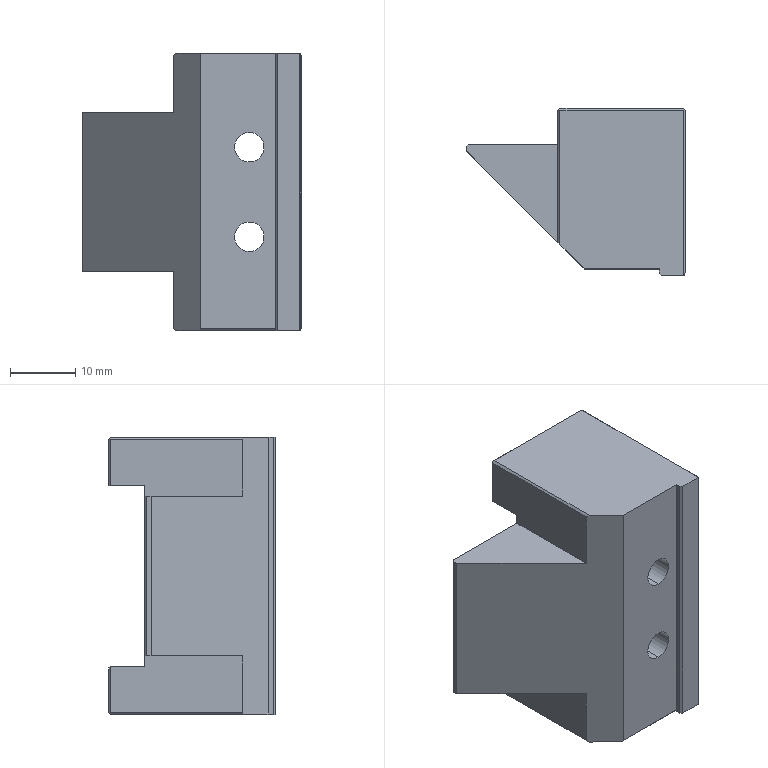Part | NX | 1 solid | 47 faces | box 33.5 x 25.5 x 42.4 mm | volume 18762 mm3 | plane 39 | cylinder 8 | commonest cylinder face diameters 4.5 x4 8 x4
STEP:
#1=CARTESIAN_POINT('',(2276.5,191.,-62.9));
#2=VERTEX_POINT('',#1);
#3=CARTESIAN_POINT('',(2265.,191.,-62.9));
#4=VERTEX_POINT('',#3);
#5=CARTESIAN_POINT('',(2270.75,191.,-62.9));
#6=DIRECTION('',(-1.,0.,0.));
#7=VECTOR('',#6,1000.);
#8=LINE('',#5,#7);
#9=EDGE_CURVE('',#2,#4,#8,.T.);
#10=ORIENTED_EDGE('',*,*,#9,.F.);
#11=CARTESIAN_POINT('',(2276.5,191.,-20.8));
#12=VERTEX_POINT('',#11);
#13=CARTESIAN_POINT('',(2276.5,191.,-19.655));
#14=DIRECTION('',(0.,0.,-1.));
#15=VECTOR('',#14,1000.);
#16=LINE('',#13,#15);
#17=EDGE_CURVE('',#12,#2,#16,.T.);
#18=ORIENTED_EDGE('',*,*,#17,.F.);
#19=CARTESIAN_POINT('',(2265.,191.,-20.8));
#20=VERTEX_POINT('',#19);
#21=CARTESIAN_POINT('',(2266.5,191.,-20.8));
#22=DIRECTION('',(1.,0.,0.));
#23=VECTOR('',#22,1000.);
#24=LINE('',#21,#23);
#25=EDGE_CURVE('',#20,#12,#24,.T.);
#26=ORIENTED_EDGE('',*,*,#25,.F.);
#27=CARTESIAN_POINT('',(2265.,191.,-42.));
#28=DIRECTION('',(0.,0.,1.));
#29=VECTOR('',#28,1000.);
#30=LINE('',#27,#29);
#31=EDGE_CURVE('',#4,#20,#30,.T.);
#32=ORIENTED_EDGE('',*,*,#31,.F.);
#33=EDGE_LOOP('',(#10,#18,#26,#32));
#34=FACE_BOUND('',#33,.T.);
#35=CARTESIAN_POINT('',(2272.5,191.,-37.4));
#36=VERTEX_POINT('',#35);
#37=CARTESIAN_POINT('',(2272.5,191.,-32.9));
#38=VERTEX_POINT('',#37);
#39=CARTESIAN_POINT('',(2272.5,191.,-35.15));
#40=DIRECTION('',(0.,1.,0.));
#41=DIRECTION('',(0.,0.,1.));
#42=AXIS2_PLACEMENT_3D('',#39,#40,#41);
#43=CIRCLE('',#42,2.25);
#44=EDGE_CURVE('',#36,#38,#43,.T.);
#45=ORIENTED_EDGE('',*,*,#44,.T.);
#46=CARTESIAN_POINT('',(2272.5,191.,-35.15));
#47=DIRECTION('',(0.,1.,0.));
#48=DIRECTION('',(0.,0.,1.));
#49=AXIS2_PLACEMENT_3D('',#46,#47,#48);
#50=CIRCLE('',#49,2.25);
#51=EDGE_CURVE('',#38,#36,#50,.T.);
#52=ORIENTED_EDGE('',*,*,#51,.T.);
#53=EDGE_LOOP('',(#45,#52));
#54=FACE_BOUND('',#53,.T.);
#55=CARTESIAN_POINT('',(2272.5,191.,-51.1));
#56=VERTEX_POINT('',#55);
#57=CARTESIAN_POINT('',(2272.5,191.,-46.6));
#58=VERTEX_POINT('',#57);
#59=CARTESIAN_POINT('',(2272.5,191.,-48.85));
#60=DIRECTION('',(0.,1.,0.));
#61=DIRECTION('',(0.,0.,1.));
#62=AXIS2_PLACEMENT_3D('',#59,#60,#61);
#63=CIRCLE('',#62,2.25);
#64=EDGE_CURVE('',#56,#58,#63,.T.);
#65=ORIENTED_EDGE('',*,*,#64,.T.);
#66=CARTESIAN_POINT('',(2272.5,191.,-48.85));
#67=DIRECTION('',(0.,1.,0.));
#68=DIRECTION('',(0.,0.,1.));
#69=AXIS2_PLACEMENT_3D('',#66,#67,#68);
#70=CIRCLE('',#69,2.25);
#71=EDGE_CURVE('',#58,#56,#70,.T.);
#72=ORIENTED_EDGE('',*,*,#71,.T.);
#73=EDGE_LOOP('',(#65,#72));
#74=FACE_BOUND('',#73,.T.);
#75=CARTESIAN_POINT('',(2261.,191.,-28.3));
#76=DIRECTION('',(0.,-1.,0.));
#77=DIRECTION('',(0.,0.,-1.));
#78=AXIS2_PLACEMENT_3D('',#75,#76,#77);
#79=PLANE('',#78);
#80=ADVANCED_FACE('',(#34,#54,#74),#79,.T.);
#81=CARTESIAN_POINT('',(2280.2,215.5,-62.9));
#82=VERTEX_POINT('',#81);
#83=CARTESIAN_POINT('',(2280.2,215.5,-56.462));
#84=VERTEX_POINT('',#83);
#85=CARTESIAN_POINT('',(2280.2,215.5,-19.655));
#86=DIRECTION('',(0.,0.,1.));
#87=VECTOR('',#86,1000.);
#88=LINE('',#85,#87);
#89=EDGE_CURVE('',#82,#84,#88,.T.);
#90=ORIENTED_EDGE('',*,*,#89,.F.);
#91=CARTESIAN_POINT('',(2261.3,215.5,-62.9));
#92=VERTEX_POINT('',#91);
#93=CARTESIAN_POINT('',(2270.75,215.5,-62.9));
#94=DIRECTION('',(-1.,0.,0.));
#95=VECTOR('',#94,1000.);
#96=LINE('',#93,#95);
#97=EDGE_CURVE('',#82,#92,#96,.T.);
#98=ORIENTED_EDGE('',*,*,#97,.T.);
#99=CARTESIAN_POINT('',(2261.3,215.5,-56.05));
#100=VERTEX_POINT('',#99);
#101=CARTESIAN_POINT('',(2261.3,215.5,-19.655));
#102=DIRECTION('',(0.,0.,1.));
#103=VECTOR('',#102,1000.);
#104=LINE('',#101,#103);
#105=EDGE_CURVE('',#92,#100,#104,.T.);
#106=ORIENTED_EDGE('',*,*,#105,.T.);
#107=CARTESIAN_POINT('',(2275.487,215.5,-56.05));
#108=VERTEX_POINT('',#107);
#109=CARTESIAN_POINT('',(2270.75,215.5,-56.05));
#110=DIRECTION('',(1.,0.,0.));
#111=VECTOR('',#110,1000.);
#112=LINE('',#109,#111);
#113=EDGE_CURVE('',#100,#108,#112,.T.);
#114=ORIENTED_EDGE('',*,*,#113,.T.);
#115=CARTESIAN_POINT('',(2279.538,215.5,-56.404));
#116=DIRECTION('',(0.9962,0.,-0.08716));
#117=VECTOR('',#116,1000.);
#118=LINE('',#115,#117);
#119=EDGE_CURVE('',#108,#84,#118,.T.);
#120=ORIENTED_EDGE('',*,*,#119,.T.);
#121=EDGE_LOOP('',(#90,#98,#106,#114,#120));
#122=FACE_BOUND('',#121,.T.);
#123=CARTESIAN_POINT('',(2266.5,215.5,-63.7));
#124=DIRECTION('',(0.,1.,0.));
#125=DIRECTION('',(0.,0.,-1.));
#126=AXIS2_PLACEMENT_3D('',#123,#124,#125);
#127=PLANE('',#126);
#128=ADVANCED_FACE('',(#122),#127,.T.);
#129=CARTESIAN_POINT('',(2247.,209.7,-54.2));
#130=VERTEX_POINT('',#129);
#131=CARTESIAN_POINT('',(2247.,209.7,-29.8));
#132=VERTEX_POINT('',#131);
#133=CARTESIAN_POINT('',(2247.,209.7,-42.));
#134=DIRECTION('',(0.,0.,1.));
#135=VECTOR('',#134,1000.);
#136=LINE('',#133,#135);
#137=EDGE_CURVE('',#130,#132,#136,.T.);
#138=ORIENTED_EDGE('',*,*,#137,.F.);
#139=CARTESIAN_POINT('',(2247.,209.,-54.2));
#140=VERTEX_POINT('',#139);
#141=CARTESIAN_POINT('',(2247.,186.964,-54.2));
#142=DIRECTION('',(0.,-1.,0.));
#143=VECTOR('',#142,1000.);
#144=LINE('',#141,#143);
#145=EDGE_CURVE('',#130,#140,#144,.T.);
#146=ORIENTED_EDGE('',*,*,#145,.T.);
#147=CARTESIAN_POINT('',(2247.,209.,-29.8));
#148=VERTEX_POINT('',#147);
#149=CARTESIAN_POINT('',(2247.,209.,-42.));
#150=DIRECTION('',(0.,0.,1.));
#151=VECTOR('',#150,1000.);
#152=LINE('',#149,#151);
#153=EDGE_CURVE('',#140,#148,#152,.T.);
#154=ORIENTED_EDGE('',*,*,#153,.T.);
#155=CARTESIAN_POINT('',(2247.,186.964,-29.8));
#156=DIRECTION('',(0.,1.,0.));
#157=VECTOR('',#156,1000.);
#158=LINE('',#155,#157);
#159=EDGE_CURVE('',#148,#132,#158,.T.);
#160=ORIENTED_EDGE('',*,*,#159,.T.);
#161=EDGE_LOOP('',(#138,#146,#154,#160));
#162=FACE_BOUND('',#161,.T.);
#163=CARTESIAN_POINT('',(2247.,203.948,-34.283));
#164=DIRECTION('',(-1.,0.,0.));
#165=DIRECTION('',(0.,0.,1.));
#166=AXIS2_PLACEMENT_3D('',#163,#164,#165);
#167=PLANE('',#166);
#168=ADVANCED_FACE('',(#162),#167,.T.);
#169=CARTESIAN_POINT('',(2275.5,210.,-28.25));
#170=VERTEX_POINT('',#169);
#171=CARTESIAN_POINT('',(2261.,210.,-28.25));
#172=VERTEX_POINT('',#171);
#173=CARTESIAN_POINT('',(2266.5,210.,-28.25));
#174=DIRECTION('',(-1.,0.,0.));
#175=VECTOR('',#174,1000.);
#176=LINE('',#173,#175);
#177=EDGE_CURVE('',#170,#172,#176,.T.);
#178=ORIENTED_EDGE('',*,*,#177,.T.);
#179=CARTESIAN_POINT('',(2261.,215.2,-28.25));
#180=VERTEX_POINT('',#179);
#181=CARTESIAN_POINT('',(2261.,186.964,-28.25));
#182=DIRECTION('',(0.,-1.,0.));
#183=VECTOR('',#182,1000.);
#184=LINE('',#181,#183);
#185=EDGE_CURVE('',#180,#172,#184,.T.);
#186=ORIENTED_EDGE('',*,*,#185,.F.);
#187=CARTESIAN_POINT('',(2261.3,215.5,-28.25));
#188=VERTEX_POINT('',#187);
#189=CARTESIAN_POINT('',(2232.764,186.964,-28.25));
#190=DIRECTION('',(0.7071,0.7071,0.));
#191=VECTOR('',#190,1000.);
#192=LINE('',#189,#191);
#193=EDGE_CURVE('',#180,#188,#192,.T.);
#194=ORIENTED_EDGE('',*,*,#193,.T.);
#195=CARTESIAN_POINT('',(2275.5,215.5,-28.25));
#196=VERTEX_POINT('',#195);
#197=CARTESIAN_POINT('',(2266.5,215.5,-28.25));
#198=DIRECTION('',(-1.,0.,0.));
#199=VECTOR('',#198,1000.);
#200=LINE('',#197,#199);
#201=EDGE_CURVE('',#196,#188,#200,.T.);
#202=ORIENTED_EDGE('',*,*,#201,.F.);
#203=CARTESIAN_POINT('',(2275.5,212.381,-28.25));
#204=DIRECTION('',(0.,-1.,0.));
#205=VECTOR('',#204,1000.);
#206=LINE('',#203,#205);
#207=EDGE_CURVE('',#196,#170,#206,.T.);
#208=ORIENTED_EDGE('',*,*,#207,.T.);
#209=EDGE_LOOP('',(#178,#186,#194,#202,#208));
#210=FACE_BOUND('',#209,.T.);
#211=CARTESIAN_POINT('',(2266.5,210.,-28.25));
#212=DIRECTION('',(0.,0.,-1.));
#213=DIRECTION('',(-1.,0.,0.));
#214=AXIS2_PLACEMENT_3D('',#211,#212,#213);
#215=PLANE('',#214);
#216=ADVANCED_FACE('',(#210),#215,.T.);
#217=ORIENTED_EDGE('',*,*,#201,.T.);
#218=CARTESIAN_POINT('',(2261.3,215.5,-21.1));
#219=VERTEX_POINT('',#218);
#220=CARTESIAN_POINT('',(2261.3,215.5,-19.655));
#221=DIRECTION('',(0.,0.,1.));
#222=VECTOR('',#221,1000.);
#223=LINE('',#220,#222);
#224=EDGE_CURVE('',#188,#219,#223,.T.);
#225=ORIENTED_EDGE('',*,*,#224,.T.);
#226=CARTESIAN_POINT('',(2280.2,215.5,-21.1));
#227=VERTEX_POINT('',#226);
#228=CARTESIAN_POINT('',(2270.75,215.5,-21.1));
#229=DIRECTION('',(1.,0.,0.));
#230=VECTOR('',#229,1000.);
#231=LINE('',#228,#230);
#232=EDGE_CURVE('',#219,#227,#231,.T.);
#233=ORIENTED_EDGE('',*,*,#232,.T.);
#234=CARTESIAN_POINT('',(2280.2,215.5,-27.839));
#235=VERTEX_POINT('',#234);
#236=CARTESIAN_POINT('',(2280.2,215.5,-19.655));
#237=DIRECTION('',(0.,0.,1.));
#238=VECTOR('',#237,1000.);
#239=LINE('',#236,#238);
#240=EDGE_CURVE('',#235,#227,#239,.T.);
#241=ORIENTED_EDGE('',*,*,#240,.F.);
#242=CARTESIAN_POINT('',(2266.5,215.5,-29.037));
#243=DIRECTION('',(-0.9962,0.,-0.08716));
#244=VECTOR('',#243,1000.);
#245=LINE('',#242,#244);
#246=EDGE_CURVE('',#235,#196,#245,.T.);
#247=ORIENTED_EDGE('',*,*,#246,.T.);
#248=EDGE_LOOP('',(#217,#225,#233,#241,#247));
#249=FACE_BOUND('',#248,.T.);
#250=CARTESIAN_POINT('',(2266.5,215.5,-28.3));
#251=DIRECTION('',(0.,1.,0.));
#252=DIRECTION('',(0.,0.,-1.));
#253=AXIS2_PLACEMENT_3D('',#250,#251,#252);
#254=PLANE('',#253);
#255=ADVANCED_FACE('',(#249),#254,.T.);
#256=CARTESIAN_POINT('',(2261.,215.2,-55.75));
#257=VERTEX_POINT('',#256);
#258=CARTESIAN_POINT('',(2275.5,215.2,-55.75));
#259=VERTEX_POINT('',#258);
#260=CARTESIAN_POINT('',(2270.75,215.2,-55.75));
#261=DIRECTION('',(1.,0.,0.));
#262=VECTOR('',#261,1000.);
#263=LINE('',#260,#262);
#264=EDGE_CURVE('',#257,#259,#263,.T.);
#265=ORIENTED_EDGE('',*,*,#264,.F.);
#266=CARTESIAN_POINT('',(2261.,210.,-55.75));
#267=VERTEX_POINT('',#266);
#268=CARTESIAN_POINT('',(2261.,186.964,-55.75));
#269=DIRECTION('',(0.,1.,0.));
#270=VECTOR('',#269,1000.);
#271=LINE('',#268,#270);
#272=EDGE_CURVE('',#267,#257,#271,.T.);
#273=ORIENTED_EDGE('',*,*,#272,.F.);
#274=CARTESIAN_POINT('',(2275.5,210.,-55.75));
#275=VERTEX_POINT('',#274);
#276=CARTESIAN_POINT('',(2266.5,210.,-55.75));
#277=DIRECTION('',(1.,0.,0.));
#278=VECTOR('',#277,1000.);
#279=LINE('',#276,#278);
#280=EDGE_CURVE('',#267,#275,#279,.T.);
#281=ORIENTED_EDGE('',*,*,#280,.T.);
#282=CARTESIAN_POINT('',(2275.5,212.381,-55.75));
#283=DIRECTION('',(0.,1.,0.));
#284=VECTOR('',#283,1000.);
#285=LINE('',#282,#284);
#286=EDGE_CURVE('',#275,#259,#285,.T.);
#287=ORIENTED_EDGE('',*,*,#286,.T.);
#288=EDGE_LOOP('',(#265,#273,#281,#287));
#289=FACE_BOUND('',#288,.T.);
#290=CARTESIAN_POINT('',(2266.5,210.65,-55.75));
#291=DIRECTION('',(0.,0.,1.));
#292=DIRECTION('',(0.,-1.,0.));
#293=AXIS2_PLACEMENT_3D('',#290,#291,#292);
#294=PLANE('',#293);
#295=ADVANCED_FACE('',(#289),#294,.T.);
#296=CARTESIAN_POINT('',(2276.5,191.3,-63.2));
#297=VERTEX_POINT('',#296);
#298=CARTESIAN_POINT('',(2264.7,191.3,-63.2));
#299=VERTEX_POINT('',#298);
#300=CARTESIAN_POINT('',(2270.75,191.3,-63.2));
#301=DIRECTION('',(-1.,0.,0.));
#302=VECTOR('',#301,1000.);
#303=LINE('',#300,#302);
#304=EDGE_CURVE('',#297,#299,#303,.T.);
#305=ORIENTED_EDGE('',*,*,#304,.T.);
#306=CARTESIAN_POINT('',(2261.3,194.7,-63.2));
#307=VERTEX_POINT('',#306);
#308=CARTESIAN_POINT('',(2266.5,189.5,-63.2));
#309=DIRECTION('',(0.7071,-0.7071,0.));
#310=VECTOR('',#309,1000.);
#311=LINE('',#308,#310);
#312=EDGE_CURVE('',#307,#299,#311,.T.);
#313=ORIENTED_EDGE('',*,*,#312,.F.);
#314=CARTESIAN_POINT('',(2261.3,215.2,-63.2));
#315=VERTEX_POINT('',#314);
#316=CARTESIAN_POINT('',(2261.3,205.1,-63.2));
#317=DIRECTION('',(0.,-1.,0.));
#318=VECTOR('',#317,1000.);
#319=LINE('',#316,#318);
#320=EDGE_CURVE('',#315,#307,#319,.T.);
#321=ORIENTED_EDGE('',*,*,#320,.F.);
#322=CARTESIAN_POINT('',(2280.2,215.2,-63.2));
#323=VERTEX_POINT('',#322);
#324=CARTESIAN_POINT('',(2270.75,215.2,-63.2));
#325=DIRECTION('',(-1.,0.,0.));
#326=VECTOR('',#325,1000.);
#327=LINE('',#324,#326);
#328=EDGE_CURVE('',#323,#315,#327,.T.);
#329=ORIENTED_EDGE('',*,*,#328,.F.);
#330=CARTESIAN_POINT('',(2280.2,190.,-63.2));
#331=VERTEX_POINT('',#330);
#332=CARTESIAN_POINT('',(2280.2,202.75,-63.2));
#333=DIRECTION('',(0.,-1.,0.));
#334=VECTOR('',#333,1000.);
#335=LINE('',#332,#334);
#336=EDGE_CURVE('',#323,#331,#335,.T.);
#337=ORIENTED_EDGE('',*,*,#336,.T.);
#338=CARTESIAN_POINT('',(2276.8,190.,-63.2));
#339=VERTEX_POINT('',#338);
#340=CARTESIAN_POINT('',(2280.5,190.,-63.2));
#341=DIRECTION('',(-1.,0.,0.));
#342=VECTOR('',#341,1000.);
#343=LINE('',#340,#342);
#344=EDGE_CURVE('',#331,#339,#343,.T.);
#345=ORIENTED_EDGE('',*,*,#344,.T.);
#346=CARTESIAN_POINT('',(2276.5,190.3,-63.2));
#347=VERTEX_POINT('',#346);
#348=CARTESIAN_POINT('',(2266.5,200.3,-63.2));
#349=DIRECTION('',(-0.7071,0.7071,0.));
#350=VECTOR('',#349,1000.);
#351=LINE('',#348,#350);
#352=EDGE_CURVE('',#339,#347,#351,.T.);
#353=ORIENTED_EDGE('',*,*,#352,.T.);
#354=CARTESIAN_POINT('',(2276.5,191.,-63.2));
#355=DIRECTION('',(0.,-1.,0.));
#356=VECTOR('',#355,1000.);
#357=LINE('',#354,#356);
#358=EDGE_CURVE('',#297,#347,#357,.T.);
#359=ORIENTED_EDGE('',*,*,#358,.F.);
#360=EDGE_LOOP('',(#305,#313,#321,#329,#337,#345,#353,#359));
#361=FACE_BOUND('',#360,.T.);
#362=CARTESIAN_POINT('',(2266.5,212.55,-63.2));
#363=DIRECTION('',(0.,0.,-1.));
#364=DIRECTION('',(0.,-1.,0.));
#365=AXIS2_PLACEMENT_3D('',#362,#363,#364);
#366=PLANE('',#365);
#367=ADVANCED_FACE('',(#361),#366,.T.);
#368=CARTESIAN_POINT('',(2276.8,190.,-20.8));
#369=VERTEX_POINT('',#368);
#370=CARTESIAN_POINT('',(2276.8,190.,-42.));
#371=DIRECTION('',(0.,0.,1.));
#372=VECTOR('',#371,1000.);
#373=LINE('',#370,#372);
#374=EDGE_CURVE('',#339,#369,#373,.T.);
#375=ORIENTED_EDGE('',*,*,#374,.F.);
#376=ORIENTED_EDGE('',*,*,#344,.F.);
#377=CARTESIAN_POINT('',(2280.2,190.,-20.8));
#378=VERTEX_POINT('',#377);
#379=CARTESIAN_POINT('',(2280.2,190.,-42.));
#380=DIRECTION('',(0.,0.,-1.));
#381=VECTOR('',#380,1000.);
#382=LINE('',#379,#381);
#383=EDGE_CURVE('',#378,#331,#382,.T.);
#384=ORIENTED_EDGE('',*,*,#383,.F.);
#385=CARTESIAN_POINT('',(2276.5,190.,-20.8));
#386=DIRECTION('',(1.,0.,0.));
#387=VECTOR('',#386,1000.);
#388=LINE('',#385,#387);
#389=EDGE_CURVE('',#369,#378,#388,.T.);
#390=ORIENTED_EDGE('',*,*,#389,.F.);
#391=EDGE_LOOP('',(#375,#376,#384,#390));
#392=FACE_BOUND('',#391,.T.);
#393=CARTESIAN_POINT('',(2263.357,190.,-43.006));
#394=DIRECTION('',(0.,-1.,0.));
#395=DIRECTION('',(0.,0.,-1.));
#396=AXIS2_PLACEMENT_3D('',#393,#394,#395);
#397=PLANE('',#396);
#398=ADVANCED_FACE('',(#392),#397,.T.);
#399=CARTESIAN_POINT('',(2272.5,210.,-44.85));
#400=VERTEX_POINT('',#399);
#401=CARTESIAN_POINT('',(2275.5,210.,-46.204));
#402=VERTEX_POINT('',#401);
#403=CARTESIAN_POINT('',(2272.5,210.,-48.85));
#404=DIRECTION('',(0.,1.,0.));
#405=DIRECTION('',(0.,0.,1.));
#406=AXIS2_PLACEMENT_3D('',#403,#404,#405);
#407=CIRCLE('',#406,4.);
#408=EDGE_CURVE('',#400,#402,#407,.T.);
#409=ORIENTED_EDGE('',*,*,#408,.T.);
#410=CARTESIAN_POINT('',(2275.5,210.,-51.496));
#411=VERTEX_POINT('',#410);
#412=CARTESIAN_POINT('',(2275.5,210.,-46.204));
#413=CARTESIAN_POINT('',(2276.9,209.878,-47.792));
#414=CARTESIAN_POINT('',(2276.9,209.878,-49.908));
#415=CARTESIAN_POINT('',(2275.5,210.,-51.496));
#416=(BOUNDED_CURVE()B_SPLINE_CURVE(3,(#412,#413,#414,#415),.UNSPECIFIED.,.F.,.F.)B_SPLINE_CURVE_WITH_KNOTS((4,4),(2.419,3.864),.UNSPECIFIED.)CURVE()GEOMETRIC_REPRESENTATION_ITEM()RATIONAL_B_SPLINE_CURVE((1.,0.8333,0.8333,1.))REPRESENTATION_ITEM(''));
#417=EDGE_CURVE('',#402,#411,#416,.T.);
#418=ORIENTED_EDGE('',*,*,#417,.T.);
#419=CARTESIAN_POINT('',(2272.5,210.,-52.85));
#420=VERTEX_POINT('',#419);
#421=CARTESIAN_POINT('',(2272.5,210.,-48.85));
#422=DIRECTION('',(0.,1.,0.));
#423=DIRECTION('',(0.,0.,1.));
#424=AXIS2_PLACEMENT_3D('',#421,#422,#423);
#425=CIRCLE('',#424,4.);
#426=EDGE_CURVE('',#411,#420,#425,.T.);
#427=ORIENTED_EDGE('',*,*,#426,.T.);
#428=CARTESIAN_POINT('',(2272.5,203.5,-52.85));
#429=VERTEX_POINT('',#428);
#430=CARTESIAN_POINT('',(2272.5,210.,-52.85));
#431=DIRECTION('',(0.,1.,0.));
#432=VECTOR('',#431,1000.);
#433=LINE('',#430,#432);
#434=EDGE_CURVE('',#420,#429,#433,.F.);
#435=ORIENTED_EDGE('',*,*,#434,.T.);
#436=CARTESIAN_POINT('',(2272.5,203.5,-44.85));
#437=VERTEX_POINT('',#436);
#438=CARTESIAN_POINT('',(2272.5,203.5,-48.85));
#439=DIRECTION('',(0.,1.,0.));
#440=DIRECTION('',(0.,0.,1.));
#441=AXIS2_PLACEMENT_3D('',#438,#439,#440);
#442=CIRCLE('',#441,4.);
#443=EDGE_CURVE('',#437,#429,#442,.T.);
#444=ORIENTED_EDGE('',*,*,#443,.F.);
#445=CARTESIAN_POINT('',(2272.5,210.,-44.85));
#446=DIRECTION('',(0.,1.,0.));
#447=VECTOR('',#446,1000.);
#448=LINE('',#445,#447);
#449=EDGE_CURVE('',#400,#437,#448,.F.);
#450=ORIENTED_EDGE('',*,*,#449,.F.);
#451=EDGE_LOOP('',(#409,#418,#427,#435,#444,#450));
#452=FACE_BOUND('',#451,.T.);
#453=CARTESIAN_POINT('',(2272.5,210.,-48.85));
#454=DIRECTION('',(0.,1.,0.));
#455=DIRECTION('',(0.,0.,1.));
#456=AXIS2_PLACEMENT_3D('',#453,#454,#455);
#457=CYLINDRICAL_SURFACE('',#456,4.);
#458=ADVANCED_FACE('',(#452),#457,.F.);
#459=CARTESIAN_POINT('',(2272.5,203.5,-48.85));
#460=DIRECTION('',(0.,1.,0.));
#461=DIRECTION('',(0.,0.,1.));
#462=AXIS2_PLACEMENT_3D('',#459,#460,#461);
#463=CIRCLE('',#462,4.);
#464=EDGE_CURVE('',#429,#437,#463,.T.);
#465=ORIENTED_EDGE('',*,*,#464,.T.);
#466=ORIENTED_EDGE('',*,*,#443,.T.);
#467=EDGE_LOOP('',(#465,#466));
#468=FACE_BOUND('',#467,.T.);
#469=CARTESIAN_POINT('',(2272.5,203.5,-51.1));
#470=VERTEX_POINT('',#469);
#471=CARTESIAN_POINT('',(2272.5,203.5,-46.6));
#472=VERTEX_POINT('',#471);
#473=CARTESIAN_POINT('',(2272.5,203.5,-48.85));
#474=DIRECTION('',(0.,1.,0.));
#475=DIRECTION('',(0.,0.,1.));
#476=AXIS2_PLACEMENT_3D('',#473,#474,#475);
#477=CIRCLE('',#476,2.25);
#478=EDGE_CURVE('',#470,#472,#477,.T.);
#479=ORIENTED_EDGE('',*,*,#478,.F.);
#480=CARTESIAN_POINT('',(2272.5,203.5,-48.85));
#481=DIRECTION('',(0.,1.,0.));
#482=DIRECTION('',(0.,0.,1.));
#483=AXIS2_PLACEMENT_3D('',#480,#481,#482);
#484=CIRCLE('',#483,2.25);
#485=EDGE_CURVE('',#472,#470,#484,.T.);
#486=ORIENTED_EDGE('',*,*,#485,.F.);
#487=EDGE_LOOP('',(#479,#486));
#488=FACE_BOUND('',#487,.T.);
#489=CARTESIAN_POINT('',(2272.5,203.5,-48.85));
#490=DIRECTION('',(0.,1.,0.));
#491=DIRECTION('',(0.,0.,-1.));
#492=AXIS2_PLACEMENT_3D('',#489,#490,#491);
#493=PLANE('',#492);
#494=ADVANCED_FACE('',(#468,#488),#493,.T.);
#495=ORIENTED_EDGE('',*,*,#478,.T.);
#496=CARTESIAN_POINT('',(2272.5,210.,-46.6));
#497=DIRECTION('',(0.,1.,0.));
#498=VECTOR('',#497,1000.);
#499=LINE('',#496,#498);
#500=EDGE_CURVE('',#58,#472,#499,.T.);
#501=ORIENTED_EDGE('',*,*,#500,.F.);
#502=ORIENTED_EDGE('',*,*,#64,.F.);
#503=CARTESIAN_POINT('',(2272.5,210.,-51.1));
#504=DIRECTION('',(0.,1.,0.));
#505=VECTOR('',#504,1000.);
#506=LINE('',#503,#505);
#507=EDGE_CURVE('',#56,#470,#506,.T.);
#508=ORIENTED_EDGE('',*,*,#507,.T.);
#509=EDGE_LOOP('',(#495,#501,#502,#508));
#510=FACE_BOUND('',#509,.T.);
#511=CARTESIAN_POINT('',(2272.5,210.,-48.85));
#512=DIRECTION('',(0.,1.,0.));
#513=DIRECTION('',(0.,0.,1.));
#514=AXIS2_PLACEMENT_3D('',#511,#512,#513);
#515=CYLINDRICAL_SURFACE('',#514,2.25);
#516=ADVANCED_FACE('',(#510),#515,.F.);
#517=CARTESIAN_POINT('',(2272.5,203.5,-37.4));
#518=VERTEX_POINT('',#517);
#519=CARTESIAN_POINT('',(2272.5,203.5,-32.9));
#520=VERTEX_POINT('',#519);
#521=CARTESIAN_POINT('',(2272.5,203.5,-35.15));
#522=DIRECTION('',(0.,1.,0.));
#523=DIRECTION('',(0.,0.,1.));
#524=AXIS2_PLACEMENT_3D('',#521,#522,#523);
#525=CIRCLE('',#524,2.25);
#526=EDGE_CURVE('',#518,#520,#525,.T.);
#527=ORIENTED_EDGE('',*,*,#526,.T.);
#528=CARTESIAN_POINT('',(2272.5,210.,-32.9));
#529=DIRECTION('',(0.,1.,0.));
#530=VECTOR('',#529,1000.);
#531=LINE('',#528,#530);
#532=EDGE_CURVE('',#38,#520,#531,.T.);
#533=ORIENTED_EDGE('',*,*,#532,.F.);
#534=ORIENTED_EDGE('',*,*,#44,.F.);
#535=CARTESIAN_POINT('',(2272.5,210.,-37.4));
#536=DIRECTION('',(0.,1.,0.));
#537=VECTOR('',#536,1000.);
#538=LINE('',#535,#537);
#539=EDGE_CURVE('',#36,#518,#538,.T.);
#540=ORIENTED_EDGE('',*,*,#539,.T.);
#541=EDGE_LOOP('',(#527,#533,#534,#540));
#542=FACE_BOUND('',#541,.T.);
#543=CARTESIAN_POINT('',(2272.5,210.,-35.15));
#544=DIRECTION('',(0.,1.,0.));
#545=DIRECTION('',(0.,0.,1.));
#546=AXIS2_PLACEMENT_3D('',#543,#544,#545);
#547=CYLINDRICAL_SURFACE('',#546,2.25);
#548=ADVANCED_FACE('',(#542),#547,.F.);
#549=CARTESIAN_POINT('',(2272.5,203.5,-39.15));
#550=VERTEX_POINT('',#549);
#551=CARTESIAN_POINT('',(2272.5,203.5,-31.15));
#552=VERTEX_POINT('',#551);
#553=CARTESIAN_POINT('',(2272.5,203.5,-35.15));
#554=DIRECTION('',(0.,1.,0.));
#555=DIRECTION('',(0.,0.,1.));
#556=AXIS2_PLACEMENT_3D('',#553,#554,#555);
#557=CIRCLE('',#556,4.);
#558=EDGE_CURVE('',#550,#552,#557,.T.);
#559=ORIENTED_EDGE('',*,*,#558,.T.);
#560=CARTESIAN_POINT('',(2272.5,203.5,-35.15));
#561=DIRECTION('',(0.,1.,0.));
#562=DIRECTION('',(0.,0.,1.));
#563=AXIS2_PLACEMENT_3D('',#560,#561,#562);
#564=CIRCLE('',#563,4.);
#565=EDGE_CURVE('',#552,#550,#564,.T.);
#566=ORIENTED_EDGE('',*,*,#565,.T.);
#567=EDGE_LOOP('',(#559,#566));
#568=FACE_BOUND('',#567,.T.);
#569=ORIENTED_EDGE('',*,*,#526,.F.);
#570=CARTESIAN_POINT('',(2272.5,203.5,-35.15));
#571=DIRECTION('',(0.,1.,0.));
#572=DIRECTION('',(0.,0.,1.));
#573=AXIS2_PLACEMENT_3D('',#570,#571,#572);
#574=CIRCLE('',#573,2.25);
#575=EDGE_CURVE('',#520,#518,#574,.T.);
#576=ORIENTED_EDGE('',*,*,#575,.F.);
#577=EDGE_LOOP('',(#569,#576));
#578=FACE_BOUND('',#577,.T.);
#579=CARTESIAN_POINT('',(2272.5,203.5,-35.15));
#580=DIRECTION('',(0.,1.,0.));
#581=DIRECTION('',(0.,0.,-1.));
#582=AXIS2_PLACEMENT_3D('',#579,#580,#581);
#583=PLANE('',#582);
#584=ADVANCED_FACE('',(#568,#578),#583,.T.);
#585=CARTESIAN_POINT('',(2272.5,210.,-31.15));
#586=VERTEX_POINT('',#585);
#587=CARTESIAN_POINT('',(2275.5,210.,-32.504));
#588=VERTEX_POINT('',#587);
#589=CARTESIAN_POINT('',(2272.5,210.,-35.15));
#590=DIRECTION('',(0.,1.,0.));
#591=DIRECTION('',(0.,0.,1.));
#592=AXIS2_PLACEMENT_3D('',#589,#590,#591);
#593=CIRCLE('',#592,4.);
#594=EDGE_CURVE('',#586,#588,#593,.T.);
#595=ORIENTED_EDGE('',*,*,#594,.T.);
#596=CARTESIAN_POINT('',(2275.5,210.,-37.796));
#597=VERTEX_POINT('',#596);
#598=CARTESIAN_POINT('',(2275.5,210.,-32.504));
#599=CARTESIAN_POINT('',(2276.9,209.878,-34.092));
#600=CARTESIAN_POINT('',(2276.9,209.878,-36.208));
#601=CARTESIAN_POINT('',(2275.5,210.,-37.796));
#602=(BOUNDED_CURVE()B_SPLINE_CURVE(3,(#598,#599,#600,#601),.UNSPECIFIED.,.F.,.F.)B_SPLINE_CURVE_WITH_KNOTS((4,4),(2.419,3.864),.UNSPECIFIED.)CURVE()GEOMETRIC_REPRESENTATION_ITEM()RATIONAL_B_SPLINE_CURVE((1.,0.8333,0.8333,1.))REPRESENTATION_ITEM(''));
#603=EDGE_CURVE('',#588,#597,#602,.T.);
#604=ORIENTED_EDGE('',*,*,#603,.T.);
#605=CARTESIAN_POINT('',(2272.5,210.,-39.15));
#606=VERTEX_POINT('',#605);
#607=CARTESIAN_POINT('',(2272.5,210.,-35.15));
#608=DIRECTION('',(0.,1.,0.));
#609=DIRECTION('',(0.,0.,1.));
#610=AXIS2_PLACEMENT_3D('',#607,#608,#609);
#611=CIRCLE('',#610,4.);
#612=EDGE_CURVE('',#597,#606,#611,.T.);
#613=ORIENTED_EDGE('',*,*,#612,.T.);
#614=CARTESIAN_POINT('',(2272.5,210.,-39.15));
#615=DIRECTION('',(0.,1.,0.));
#616=VECTOR('',#615,1000.);
#617=LINE('',#614,#616);
#618=EDGE_CURVE('',#606,#550,#617,.F.);
#619=ORIENTED_EDGE('',*,*,#618,.T.);
#620=ORIENTED_EDGE('',*,*,#565,.F.);
#621=CARTESIAN_POINT('',(2272.5,210.,-31.15));
#622=DIRECTION('',(0.,1.,0.));
#623=VECTOR('',#622,1000.);
#624=LINE('',#621,#623);
#625=EDGE_CURVE('',#586,#552,#624,.F.);
#626=ORIENTED_EDGE('',*,*,#625,.F.);
#627=EDGE_LOOP('',(#595,#604,#613,#619,#620,#626));
#628=FACE_BOUND('',#627,.T.);
#629=CARTESIAN_POINT('',(2272.5,210.,-35.15));
#630=DIRECTION('',(0.,1.,0.));
#631=DIRECTION('',(0.,0.,1.));
#632=AXIS2_PLACEMENT_3D('',#629,#630,#631);
#633=CYLINDRICAL_SURFACE('',#632,4.);
#634=ADVANCED_FACE('',(#628),#633,.F.);
#635=ORIENTED_EDGE('',*,*,#17,.T.);
#636=CARTESIAN_POINT('',(2276.5,186.964,-58.864));
#637=DIRECTION('',(0.,0.7071,-0.7071));
#638=VECTOR('',#637,1000.);
#639=LINE('',#636,#638);
#640=EDGE_CURVE('',#2,#297,#639,.T.);
#641=ORIENTED_EDGE('',*,*,#640,.T.);
#642=ORIENTED_EDGE('',*,*,#358,.T.);
#643=CARTESIAN_POINT('',(2276.5,190.3,-20.8));
#644=VERTEX_POINT('',#643);
#645=CARTESIAN_POINT('',(2276.5,190.3,-42.));
#646=DIRECTION('',(0.,0.,1.));
#647=VECTOR('',#646,1000.);
#648=LINE('',#645,#647);
#649=EDGE_CURVE('',#347,#644,#648,.T.);
#650=ORIENTED_EDGE('',*,*,#649,.T.);
#651=CARTESIAN_POINT('',(2276.5,191.,-20.8));
#652=DIRECTION('',(0.,-1.,0.));
#653=VECTOR('',#652,1000.);
#654=LINE('',#651,#653);
#655=EDGE_CURVE('',#12,#644,#654,.T.);
#656=ORIENTED_EDGE('',*,*,#655,.F.);
#657=EDGE_LOOP('',(#635,#641,#642,#650,#656));
#658=FACE_BOUND('',#657,.T.);
#659=CARTESIAN_POINT('',(2276.5,191.,-63.2));
#660=DIRECTION('',(-1.,0.,0.));
#661=DIRECTION('',(0.,0.,1.));
#662=AXIS2_PLACEMENT_3D('',#659,#660,#661);
#663=PLANE('',#662);
#664=ADVANCED_FACE('',(#658),#663,.T.);
#665=CARTESIAN_POINT('',(2261.3,215.2,-20.8));
#666=VERTEX_POINT('',#665);
#667=CARTESIAN_POINT('',(2280.2,215.2,-20.8));
#668=VERTEX_POINT('',#667);
#669=CARTESIAN_POINT('',(2270.75,215.2,-20.8));
#670=DIRECTION('',(1.,0.,0.));
#671=VECTOR('',#670,1000.);
#672=LINE('',#669,#671);
#673=EDGE_CURVE('',#666,#668,#672,.T.);
#674=ORIENTED_EDGE('',*,*,#673,.F.);
#675=CARTESIAN_POINT('',(2261.3,194.7,-20.8));
#676=VERTEX_POINT('',#675);
#677=CARTESIAN_POINT('',(2261.3,205.1,-20.8));
#678=DIRECTION('',(0.,1.,0.));
#679=VECTOR('',#678,1000.);
#680=LINE('',#677,#679);
#681=EDGE_CURVE('',#676,#666,#680,.T.);
#682=ORIENTED_EDGE('',*,*,#681,.F.);
#683=CARTESIAN_POINT('',(2266.5,189.5,-20.8));
#684=DIRECTION('',(-0.7071,0.7071,0.));
#685=VECTOR('',#684,1000.);
#686=LINE('',#683,#685);
#687=EDGE_CURVE('',#20,#676,#686,.T.);
#688=ORIENTED_EDGE('',*,*,#687,.F.);
#689=ORIENTED_EDGE('',*,*,#25,.T.);
#690=ORIENTED_EDGE('',*,*,#655,.T.);
#691=CARTESIAN_POINT('',(2266.5,200.3,-20.8));
#692=DIRECTION('',(0.7071,-0.7071,0.));
#693=VECTOR('',#692,1000.);
#694=LINE('',#691,#693);
#695=EDGE_CURVE('',#644,#369,#694,.T.);
#696=ORIENTED_EDGE('',*,*,#695,.T.);
#697=ORIENTED_EDGE('',*,*,#389,.T.);
#698=CARTESIAN_POINT('',(2280.2,202.9,-20.8));
#699=DIRECTION('',(0.,-1.,0.));
#700=VECTOR('',#699,1000.);
#701=LINE('',#698,#700);
#702=EDGE_CURVE('',#668,#378,#701,.T.);
#703=ORIENTED_EDGE('',*,*,#702,.F.);
#704=EDGE_LOOP('',(#674,#682,#688,#689,#690,#696,#697,#703));
#705=FACE_BOUND('',#704,.T.);
#706=CARTESIAN_POINT('',(2276.5,191.,-20.8));
#707=DIRECTION('',(0.,0.,1.));
#708=DIRECTION('',(1.,0.,0.));
#709=AXIS2_PLACEMENT_3D('',#706,#707,#708);
#710=PLANE('',#709);
#711=ADVANCED_FACE('',(#705),#710,.T.);
#712=ORIENTED_EDGE('',*,*,#159,.F.);
#713=CARTESIAN_POINT('',(2261.,195.,-29.8));
#714=VERTEX_POINT('',#713);
#715=CARTESIAN_POINT('',(2266.5,189.5,-29.8));
#716=DIRECTION('',(-0.7071,0.7071,0.));
#717=VECTOR('',#716,1000.);
#718=LINE('',#715,#717);
#719=EDGE_CURVE('',#714,#148,#718,.T.);
#720=ORIENTED_EDGE('',*,*,#719,.F.);
#721=CARTESIAN_POINT('',(2261.,210.,-29.8));
#722=VERTEX_POINT('',#721);
#723=CARTESIAN_POINT('',(2261.,186.964,-29.8));
#724=DIRECTION('',(0.,1.,0.));
#725=VECTOR('',#724,1000.);
#726=LINE('',#723,#725);
#727=EDGE_CURVE('',#714,#722,#726,.T.);
#728=ORIENTED_EDGE('',*,*,#727,.T.);
#729=CARTESIAN_POINT('',(2247.3,210.,-29.8));
#730=VERTEX_POINT('',#729);
#731=CARTESIAN_POINT('',(2266.5,210.,-29.8));
#732=DIRECTION('',(1.,0.,0.));
#733=VECTOR('',#732,1000.);
#734=LINE('',#731,#733);
#735=EDGE_CURVE('',#730,#722,#734,.T.);
#736=ORIENTED_EDGE('',*,*,#735,.F.);
#737=CARTESIAN_POINT('',(2266.5,229.2,-29.8));
#738=DIRECTION('',(-0.7071,-0.7071,0.));
#739=VECTOR('',#738,1000.);
#740=LINE('',#737,#739);
#741=EDGE_CURVE('',#730,#132,#740,.T.);
#742=ORIENTED_EDGE('',*,*,#741,.T.);
#743=EDGE_LOOP('',(#712,#720,#728,#736,#742));
#744=FACE_BOUND('',#743,.T.);
#745=CARTESIAN_POINT('',(2261.,210.,-29.8));
#746=DIRECTION('',(0.,0.,1.));
#747=DIRECTION('',(1.,0.,0.));
#748=AXIS2_PLACEMENT_3D('',#745,#746,#747);
#749=PLANE('',#748);
#750=ADVANCED_FACE('',(#744),#749,.T.);
#751=ORIENTED_EDGE('',*,*,#177,.F.);
#752=CARTESIAN_POINT('',(2275.5,210.,-19.655));
#753=DIRECTION('',(0.,0.,-1.));
#754=VECTOR('',#753,1000.);
#755=LINE('',#752,#754);
#756=EDGE_CURVE('',#170,#588,#755,.T.);
#757=ORIENTED_EDGE('',*,*,#756,.T.);
#758=ORIENTED_EDGE('',*,*,#594,.F.);
#759=CARTESIAN_POINT('',(2272.5,210.,-35.15));
#760=DIRECTION('',(0.,1.,0.));
#761=DIRECTION('',(0.,0.,1.));
#762=AXIS2_PLACEMENT_3D('',#759,#760,#761);
#763=CIRCLE('',#762,4.);
#764=EDGE_CURVE('',#606,#586,#763,.T.);
#765=ORIENTED_EDGE('',*,*,#764,.F.);
#766=ORIENTED_EDGE('',*,*,#612,.F.);
#767=CARTESIAN_POINT('',(2275.5,210.,-19.655));
#768=DIRECTION('',(0.,0.,-1.));
#769=VECTOR('',#768,1000.);
#770=LINE('',#767,#769);
#771=EDGE_CURVE('',#597,#402,#770,.T.);
#772=ORIENTED_EDGE('',*,*,#771,.T.);
#773=ORIENTED_EDGE('',*,*,#408,.F.);
#774=CARTESIAN_POINT('',(2272.5,210.,-48.85));
#775=DIRECTION('',(0.,1.,0.));
#776=DIRECTION('',(0.,0.,1.));
#777=AXIS2_PLACEMENT_3D('',#774,#775,#776);
#778=CIRCLE('',#777,4.);
#779=EDGE_CURVE('',#420,#400,#778,.T.);
#780=ORIENTED_EDGE('',*,*,#779,.F.);
#781=ORIENTED_EDGE('',*,*,#426,.F.);
#782=CARTESIAN_POINT('',(2275.5,210.,-19.655));
#783=DIRECTION('',(0.,0.,-1.));
#784=VECTOR('',#783,1000.);
#785=LINE('',#782,#784);
#786=EDGE_CURVE('',#411,#275,#785,.T.);
#787=ORIENTED_EDGE('',*,*,#786,.T.);
#788=ORIENTED_EDGE('',*,*,#280,.F.);
#789=CARTESIAN_POINT('',(2261.,210.,-54.2));
#790=VERTEX_POINT('',#789);
#791=CARTESIAN_POINT('',(2261.,210.,-19.655));
#792=DIRECTION('',(0.,0.,-1.));
#793=VECTOR('',#792,1000.);
#794=LINE('',#791,#793);
#795=EDGE_CURVE('',#790,#267,#794,.T.);
#796=ORIENTED_EDGE('',*,*,#795,.F.);
#797=CARTESIAN_POINT('',(2247.3,210.,-54.2));
#798=VERTEX_POINT('',#797);
#799=CARTESIAN_POINT('',(2266.5,210.,-54.2));
#800=DIRECTION('',(-1.,0.,0.));
#801=VECTOR('',#800,1000.);
#802=LINE('',#799,#801);
#803=EDGE_CURVE('',#790,#798,#802,.T.);
#804=ORIENTED_EDGE('',*,*,#803,.T.);
#805=CARTESIAN_POINT('',(2247.3,210.,-42.));
#806=DIRECTION('',(0.,0.,1.));
#807=VECTOR('',#806,1000.);
#808=LINE('',#805,#807);
#809=EDGE_CURVE('',#798,#730,#808,.T.);
#810=ORIENTED_EDGE('',*,*,#809,.T.);
#811=ORIENTED_EDGE('',*,*,#735,.T.);
#812=CARTESIAN_POINT('',(2261.,210.,-19.655));
#813=DIRECTION('',(0.,0.,1.));
#814=VECTOR('',#813,1000.);
#815=LINE('',#812,#814);
#816=EDGE_CURVE('',#722,#172,#815,.T.);
#817=ORIENTED_EDGE('',*,*,#816,.T.);
#818=EDGE_LOOP('',(#751,#757,#758,#765,#766,#772,#773,#780,#781,#787,#788,#796,#804,#810,#811,#817));
#819=FACE_BOUND('',#818,.T.);
#820=CARTESIAN_POINT('',(2261.,210.,-55.7));
#821=DIRECTION('',(0.,1.,0.));
#822=DIRECTION('',(1.,0.,0.));
#823=AXIS2_PLACEMENT_3D('',#820,#821,#822);
#824=PLANE('',#823);
#825=ADVANCED_FACE('',(#819),#824,.T.);
#826=CARTESIAN_POINT('',(2261.,195.,-54.2));
#827=VERTEX_POINT('',#826);
#828=CARTESIAN_POINT('',(2261.,186.964,-54.2));
#829=DIRECTION('',(0.,-1.,0.));
#830=VECTOR('',#829,1000.);
#831=LINE('',#828,#830);
#832=EDGE_CURVE('',#790,#827,#831,.T.);
#833=ORIENTED_EDGE('',*,*,#832,.T.);
#834=CARTESIAN_POINT('',(2266.5,189.5,-54.2));
#835=DIRECTION('',(0.7071,-0.7071,0.));
#836=VECTOR('',#835,1000.);
#837=LINE('',#834,#836);
#838=EDGE_CURVE('',#140,#827,#837,.T.);
#839=ORIENTED_EDGE('',*,*,#838,.F.);
#840=ORIENTED_EDGE('',*,*,#145,.F.);
#841=CARTESIAN_POINT('',(2266.5,229.2,-54.2));
#842=DIRECTION('',(0.7071,0.7071,0.));
#843=VECTOR('',#842,1000.);
#844=LINE('',#841,#843);
#845=EDGE_CURVE('',#130,#798,#844,.T.);
#846=ORIENTED_EDGE('',*,*,#845,.T.);
#847=ORIENTED_EDGE('',*,*,#803,.F.);
#848=EDGE_LOOP('',(#833,#839,#840,#846,#847));
#849=FACE_BOUND('',#848,.T.);
#850=CARTESIAN_POINT('',(2261.,191.,-54.2));
#851=DIRECTION('',(0.,0.,-1.));
#852=DIRECTION('',(0.,-1.,0.));
#853=AXIS2_PLACEMENT_3D('',#850,#851,#852);
#854=PLANE('',#853);
#855=ADVANCED_FACE('',(#849),#854,.T.);
#856=ORIENTED_EDGE('',*,*,#153,.F.);
#857=ORIENTED_EDGE('',*,*,#838,.T.);
#858=CARTESIAN_POINT('',(2261.,195.,-62.9));
#859=VERTEX_POINT('',#858);
#860=CARTESIAN_POINT('',(2261.,195.,-19.655));
#861=DIRECTION('',(0.,0.,-1.));
#862=VECTOR('',#861,1000.);
#863=LINE('',#860,#862);
#864=EDGE_CURVE('',#827,#859,#863,.T.);
#865=ORIENTED_EDGE('',*,*,#864,.T.);
#866=CARTESIAN_POINT('',(2266.5,189.5,-68.4));
#867=DIRECTION('',(-0.5774,0.5774,0.5774));
#868=VECTOR('',#867,1000.);
#869=LINE('',#866,#868);
#870=EDGE_CURVE('',#307,#859,#869,.T.);
#871=ORIENTED_EDGE('',*,*,#870,.F.);
#872=ORIENTED_EDGE('',*,*,#312,.T.);
#873=CARTESIAN_POINT('',(2269.036,186.964,-58.864));
#874=DIRECTION('',(-0.5774,0.5774,-0.5774));
#875=VECTOR('',#874,1000.);
#876=LINE('',#873,#875);
#877=EDGE_CURVE('',#4,#299,#876,.T.);
#878=ORIENTED_EDGE('',*,*,#877,.F.);
#879=ORIENTED_EDGE('',*,*,#31,.T.);
#880=ORIENTED_EDGE('',*,*,#687,.T.);
#881=CARTESIAN_POINT('',(2261.,195.,-21.1));
#882=VERTEX_POINT('',#881);
#883=CARTESIAN_POINT('',(2266.5,189.5,-15.6));
#884=DIRECTION('',(0.5774,-0.5774,0.5774));
#885=VECTOR('',#884,1000.);
#886=LINE('',#883,#885);
#887=EDGE_CURVE('',#882,#676,#886,.T.);
#888=ORIENTED_EDGE('',*,*,#887,.F.);
#889=CARTESIAN_POINT('',(2261.,195.,-19.655));
#890=DIRECTION('',(0.,0.,-1.));
#891=VECTOR('',#890,1000.);
#892=LINE('',#889,#891);
#893=EDGE_CURVE('',#882,#714,#892,.T.);
#894=ORIENTED_EDGE('',*,*,#893,.T.);
#895=ORIENTED_EDGE('',*,*,#719,.T.);
#896=EDGE_LOOP('',(#856,#857,#865,#871,#872,#878,#879,#880,#888,#894,#895));
#897=FACE_BOUND('',#896,.T.);
#898=CARTESIAN_POINT('',(2256.,200.,-42.));
#899=DIRECTION('',(-0.7071,-0.7071,0.));
#900=DIRECTION('',(-0.7071,0.7071,0.));
#901=AXIS2_PLACEMENT_3D('',#898,#899,#900);
#902=PLANE('',#901);
#903=ADVANCED_FACE('',(#897),#902,.T.);
#904=ORIENTED_EDGE('',*,*,#97,.F.);
#905=CARTESIAN_POINT('',(2280.35,215.35,-63.05));
#906=VERTEX_POINT('',#905);
#907=CARTESIAN_POINT('',(2308.736,186.964,-91.436));
#908=DIRECTION('',(-0.5774,0.5774,0.5774));
#909=VECTOR('',#908,1000.);
#910=LINE('',#907,#909);
#911=EDGE_CURVE('',#906,#82,#910,.T.);
#912=ORIENTED_EDGE('',*,*,#911,.F.);
#913=CARTESIAN_POINT('',(2251.964,186.964,-91.436));
#914=DIRECTION('',(0.5774,0.5774,0.5774));
#915=VECTOR('',#914,1000.);
#916=LINE('',#913,#915);
#917=EDGE_CURVE('',#323,#906,#916,.T.);
#918=ORIENTED_EDGE('',*,*,#917,.F.);
#919=ORIENTED_EDGE('',*,*,#328,.T.);
#920=CARTESIAN_POINT('',(2261.15,215.35,-63.05));
#921=VERTEX_POINT('',#920);
#922=CARTESIAN_POINT('',(2289.536,186.964,-91.436));
#923=DIRECTION('',(0.5774,-0.5774,-0.5774));
#924=VECTOR('',#923,1000.);
#925=LINE('',#922,#924);
#926=EDGE_CURVE('',#921,#315,#925,.T.);
#927=ORIENTED_EDGE('',*,*,#926,.F.);
#928=CARTESIAN_POINT('',(2232.764,186.964,-91.436));
#929=DIRECTION('',(0.5774,0.5774,0.5774));
#930=VECTOR('',#929,1000.);
#931=LINE('',#928,#930);
#932=EDGE_CURVE('',#921,#92,#931,.T.);
#933=ORIENTED_EDGE('',*,*,#932,.T.);
#934=EDGE_LOOP('',(#904,#912,#918,#919,#927,#933));
#935=FACE_BOUND('',#934,.T.);
#936=CARTESIAN_POINT('',(2270.75,215.35,-63.05));
#937=DIRECTION('',(0.,0.7071,-0.7071));
#938=DIRECTION('',(-1.,0.,0.));
#939=AXIS2_PLACEMENT_3D('',#936,#937,#938);
#940=PLANE('',#939);
#941=ADVANCED_FACE('',(#935),#940,.T.);
#942=CARTESIAN_POINT('',(2280.288,190.088,-20.888));
#943=VERTEX_POINT('',#942);
#944=CARTESIAN_POINT('',(2280.288,190.088,-63.112));
#945=VERTEX_POINT('',#944);
#946=CARTESIAN_POINT('',(2280.288,190.088,-42.));
#947=DIRECTION('',(0.,0.,-1.));
#948=VECTOR('',#947,1000.);
#949=LINE('',#946,#948);
#950=EDGE_CURVE('',#943,#945,#949,.T.);
#951=ORIENTED_EDGE('',*,*,#950,.F.);
#952=CARTESIAN_POINT('',(2266.5,176.3,-7.1));
#953=DIRECTION('',(-0.5774,-0.5774,0.5774));
#954=VECTOR('',#953,1000.);
#955=LINE('',#952,#954);
#956=EDGE_CURVE('',#943,#378,#955,.T.);
#957=ORIENTED_EDGE('',*,*,#956,.T.);
#958=ORIENTED_EDGE('',*,*,#383,.T.);
#959=CARTESIAN_POINT('',(2323.745,233.545,-19.655));
#960=DIRECTION('',(-0.5774,-0.5774,-0.5774));
#961=VECTOR('',#960,1000.);
#962=LINE('',#959,#961);
#963=EDGE_CURVE('',#945,#331,#962,.T.);
#964=ORIENTED_EDGE('',*,*,#963,.F.);
#965=EDGE_LOOP('',(#951,#957,#958,#964));
#966=FACE_BOUND('',#965,.T.);
#967=CARTESIAN_POINT('',(2280.35,190.15,-42.));
#968=DIRECTION('',(-0.7071,0.7071,0.));
#969=DIRECTION('',(0.,0.,1.));
#970=AXIS2_PLACEMENT_3D('',#967,#968,#969);
#971=PLANE('',#970);
#972=ADVANCED_FACE('',(#966),#971,.F.);
#973=ORIENTED_EDGE('',*,*,#304,.F.);
#974=ORIENTED_EDGE('',*,*,#640,.F.);
#975=ORIENTED_EDGE('',*,*,#9,.T.);
#976=ORIENTED_EDGE('',*,*,#877,.T.);
#977=EDGE_LOOP('',(#973,#974,#975,#976));
#978=FACE_BOUND('',#977,.T.);
#979=CARTESIAN_POINT('',(2270.75,191.15,-63.05));
#980=DIRECTION('',(0.,-0.7071,-0.7071));
#981=DIRECTION('',(0.,-0.7071,0.7071));
#982=AXIS2_PLACEMENT_3D('',#979,#980,#981);
#983=PLANE('',#982);
#984=ADVANCED_FACE('',(#978),#983,.T.);
#985=ORIENTED_EDGE('',*,*,#673,.T.);
#986=CARTESIAN_POINT('',(2280.35,215.35,-20.95));
#987=VERTEX_POINT('',#986);
#988=CARTESIAN_POINT('',(2251.964,186.964,7.436));
#989=DIRECTION('',(-0.5774,-0.5774,0.5774));
#990=VECTOR('',#989,1000.);
#991=LINE('',#988,#990);
#992=EDGE_CURVE('',#987,#668,#991,.T.);
#993=ORIENTED_EDGE('',*,*,#992,.F.);
#994=CARTESIAN_POINT('',(2266.5,229.2,-34.8));
#995=DIRECTION('',(-0.5774,0.5774,-0.5774));
#996=VECTOR('',#995,1000.);
#997=LINE('',#994,#996);
#998=EDGE_CURVE('',#987,#227,#997,.T.);
#999=ORIENTED_EDGE('',*,*,#998,.T.);
#1000=ORIENTED_EDGE('',*,*,#232,.F.);
#1001=CARTESIAN_POINT('',(2261.15,215.35,-20.95));
#1002=VERTEX_POINT('',#1001);
#1003=CARTESIAN_POINT('',(2232.764,186.964,7.436));
#1004=DIRECTION('',(0.5774,0.5774,-0.5774));
#1005=VECTOR('',#1004,1000.);
#1006=LINE('',#1003,#1005);
#1007=EDGE_CURVE('',#1002,#219,#1006,.T.);
#1008=ORIENTED_EDGE('',*,*,#1007,.F.);
#1009=CARTESIAN_POINT('',(2289.536,186.964,7.436));
#1010=DIRECTION('',(0.5774,-0.5774,0.5774));
#1011=VECTOR('',#1010,1000.);
#1012=LINE('',#1009,#1011);
#1013=EDGE_CURVE('',#1002,#666,#1012,.T.);
#1014=ORIENTED_EDGE('',*,*,#1013,.T.);
#1015=EDGE_LOOP('',(#985,#993,#999,#1000,#1008,#1014));
#1016=FACE_BOUND('',#1015,.T.);
#1017=CARTESIAN_POINT('',(2270.75,215.35,-20.95));
#1018=DIRECTION('',(0.,-0.7071,-0.7071));
#1019=DIRECTION('',(0.,-0.7071,0.7071));
#1020=AXIS2_PLACEMENT_3D('',#1017,#1018,#1019);
#1021=PLANE('',#1020);
#1022=ADVANCED_FACE('',(#1016),#1021,.F.);
#1023=ORIENTED_EDGE('',*,*,#137,.T.);
#1024=ORIENTED_EDGE('',*,*,#741,.F.);
#1025=ORIENTED_EDGE('',*,*,#809,.F.);
#1026=ORIENTED_EDGE('',*,*,#845,.F.);
#1027=EDGE_LOOP('',(#1023,#1024,#1025,#1026));
#1028=FACE_BOUND('',#1027,.T.);
#1029=CARTESIAN_POINT('',(2247.15,209.85,-42.));
#1030=DIRECTION('',(0.7071,-0.7071,0.));
#1031=DIRECTION('',(0.,0.,-1.));
#1032=AXIS2_PLACEMENT_3D('',#1029,#1030,#1031);
#1033=PLANE('',#1032);
#1034=ADVANCED_FACE('',(#1028),#1033,.F.);
#1035=ORIENTED_EDGE('',*,*,#374,.T.);
#1036=ORIENTED_EDGE('',*,*,#695,.F.);
#1037=ORIENTED_EDGE('',*,*,#649,.F.);
#1038=ORIENTED_EDGE('',*,*,#352,.F.);
#1039=EDGE_LOOP('',(#1035,#1036,#1037,#1038));
#1040=FACE_BOUND('',#1039,.T.);
#1041=CARTESIAN_POINT('',(2276.65,190.15,-42.));
#1042=DIRECTION('',(0.7071,0.7071,0.));
#1043=DIRECTION('',(0.,0.,-1.));
#1044=AXIS2_PLACEMENT_3D('',#1041,#1042,#1043);
#1045=PLANE('',#1044);
#1046=ADVANCED_FACE('',(#1040),#1045,.F.);
#1047=ORIENTED_EDGE('',*,*,#950,.T.);
#1048=CARTESIAN_POINT('',(2280.5,190.6,-62.9));
#1049=VERTEX_POINT('',#1048);
#1050=CARTESIAN_POINT('',(2278.994,186.964,-64.406));
#1051=DIRECTION('',(0.3574,0.8629,0.3574));
#1052=VECTOR('',#1051,1000.);
#1053=LINE('',#1050,#1052);
#1054=EDGE_CURVE('',#945,#1049,#1053,.T.);
#1055=ORIENTED_EDGE('',*,*,#1054,.T.);
#1056=CARTESIAN_POINT('',(2280.5,190.6,-21.1));
#1057=VERTEX_POINT('',#1056);
#1058=CARTESIAN_POINT('',(2280.5,190.6,-42.));
#1059=DIRECTION('',(0.,0.,-1.));
#1060=VECTOR('',#1059,1000.);
#1061=LINE('',#1058,#1060);
#1062=EDGE_CURVE('',#1057,#1049,#1061,.T.);
#1063=ORIENTED_EDGE('',*,*,#1062,.F.);
#1064=CARTESIAN_POINT('',(2278.994,186.964,-19.594));
#1065=DIRECTION('',(0.3574,0.8629,-0.3574));
#1066=VECTOR('',#1065,1000.);
#1067=LINE('',#1064,#1066);
#1068=EDGE_CURVE('',#943,#1057,#1067,.T.);
#1069=ORIENTED_EDGE('',*,*,#1068,.F.);
#1070=EDGE_LOOP('',(#1047,#1055,#1063,#1069));
#1071=FACE_BOUND('',#1070,.T.);
#1072=CARTESIAN_POINT('',(2280.394,190.344,-42.));
#1073=DIRECTION('',(-0.9239,0.3827,0.));
#1074=DIRECTION('',(0.,0.,1.));
#1075=AXIS2_PLACEMENT_3D('',#1072,#1073,#1074);
#1076=PLANE('',#1075);
#1077=ADVANCED_FACE('',(#1071),#1076,.F.);
#1078=ORIENTED_EDGE('',*,*,#264,.T.);
#1079=CARTESIAN_POINT('',(2276.733,186.964,-27.514));
#1080=DIRECTION('',(0.03086,-0.7068,0.7068));
#1081=VECTOR('',#1080,1000.);
#1082=LINE('',#1079,#1081);
#1083=EDGE_CURVE('',#108,#259,#1082,.T.);
#1084=ORIENTED_EDGE('',*,*,#1083,.F.);
#1085=ORIENTED_EDGE('',*,*,#113,.F.);
#1086=CARTESIAN_POINT('',(2232.764,186.964,-27.514));
#1087=DIRECTION('',(-0.5774,-0.5774,0.5774));
#1088=VECTOR('',#1087,1000.);
#1089=LINE('',#1086,#1088);
#1090=EDGE_CURVE('',#100,#257,#1089,.T.);
#1091=ORIENTED_EDGE('',*,*,#1090,.T.);
#1092=EDGE_LOOP('',(#1078,#1084,#1085,#1091));
#1093=FACE_BOUND('',#1092,.T.);
#1094=CARTESIAN_POINT('',(2270.75,215.35,-55.9));
#1095=DIRECTION('',(0.,-0.7071,-0.7071));
#1096=DIRECTION('',(0.,-0.7071,0.7071));
#1097=AXIS2_PLACEMENT_3D('',#1094,#1095,#1096);
#1098=PLANE('',#1097);
#1099=ADVANCED_FACE('',(#1093),#1098,.F.);
#1100=ORIENTED_EDGE('',*,*,#558,.F.);
#1101=ORIENTED_EDGE('',*,*,#618,.F.);
#1102=ORIENTED_EDGE('',*,*,#764,.T.);
#1103=ORIENTED_EDGE('',*,*,#625,.T.);
#1104=EDGE_LOOP('',(#1100,#1101,#1102,#1103));
#1105=FACE_BOUND('',#1104,.T.);
#1106=CARTESIAN_POINT('',(2272.5,210.,-35.15));
#1107=DIRECTION('',(0.,1.,0.));
#1108=DIRECTION('',(0.,0.,1.));
#1109=AXIS2_PLACEMENT_3D('',#1106,#1107,#1108);
#1110=CYLINDRICAL_SURFACE('',#1109,4.);
#1111=ADVANCED_FACE('',(#1105),#1110,.F.);
#1112=ORIENTED_EDGE('',*,*,#500,.T.);
#1113=ORIENTED_EDGE('',*,*,#485,.T.);
#1114=ORIENTED_EDGE('',*,*,#507,.F.);
#1115=ORIENTED_EDGE('',*,*,#71,.F.);
#1116=EDGE_LOOP('',(#1112,#1113,#1114,#1115));
#1117=FACE_BOUND('',#1116,.T.);
#1118=CARTESIAN_POINT('',(2272.5,210.,-48.85));
#1119=DIRECTION('',(0.,1.,0.));
#1120=DIRECTION('',(0.,0.,1.));
#1121=AXIS2_PLACEMENT_3D('',#1118,#1119,#1120);
#1122=CYLINDRICAL_SURFACE('',#1121,2.25);
#1123=ADVANCED_FACE('',(#1117),#1122,.F.);
#1124=ORIENTED_EDGE('',*,*,#464,.F.);
#1125=ORIENTED_EDGE('',*,*,#434,.F.);
#1126=ORIENTED_EDGE('',*,*,#779,.T.);
#1127=ORIENTED_EDGE('',*,*,#449,.T.);
#1128=EDGE_LOOP('',(#1124,#1125,#1126,#1127));
#1129=FACE_BOUND('',#1128,.T.);
#1130=CARTESIAN_POINT('',(2272.5,210.,-48.85));
#1131=DIRECTION('',(0.,1.,0.));
#1132=DIRECTION('',(0.,0.,1.));
#1133=AXIS2_PLACEMENT_3D('',#1130,#1131,#1132);
#1134=CYLINDRICAL_SURFACE('',#1133,4.);
#1135=ADVANCED_FACE('',(#1129),#1134,.F.);
#1136=ORIENTED_EDGE('',*,*,#532,.T.);
#1137=ORIENTED_EDGE('',*,*,#575,.T.);
#1138=ORIENTED_EDGE('',*,*,#539,.F.);
#1139=ORIENTED_EDGE('',*,*,#51,.F.);
#1140=EDGE_LOOP('',(#1136,#1137,#1138,#1139));
#1141=FACE_BOUND('',#1140,.T.);
#1142=CARTESIAN_POINT('',(2272.5,210.,-35.15));
#1143=DIRECTION('',(0.,1.,0.));
#1144=DIRECTION('',(0.,0.,1.));
#1145=AXIS2_PLACEMENT_3D('',#1142,#1143,#1144);
#1146=CYLINDRICAL_SURFACE('',#1145,2.25);
#1147=ADVANCED_FACE('',(#1141),#1146,.F.);
#1148=CARTESIAN_POINT('',(2261.,215.2,-62.9));
#1149=VERTEX_POINT('',#1148);
#1150=CARTESIAN_POINT('',(2261.,205.1,-62.9));
#1151=DIRECTION('',(0.,-1.,0.));
#1152=VECTOR('',#1151,1000.);
#1153=LINE('',#1150,#1152);
#1154=EDGE_CURVE('',#1149,#859,#1153,.T.);
#1155=ORIENTED_EDGE('',*,*,#1154,.T.);
#1156=ORIENTED_EDGE('',*,*,#864,.F.);
#1157=ORIENTED_EDGE('',*,*,#832,.F.);
#1158=ORIENTED_EDGE('',*,*,#795,.T.);
#1159=ORIENTED_EDGE('',*,*,#272,.T.);
#1160=CARTESIAN_POINT('',(2261.,215.2,-19.655));
#1161=DIRECTION('',(0.,0.,1.));
#1162=VECTOR('',#1161,1000.);
#1163=LINE('',#1160,#1162);
#1164=EDGE_CURVE('',#1149,#257,#1163,.T.);
#1165=ORIENTED_EDGE('',*,*,#1164,.F.);
#1166=EDGE_LOOP('',(#1155,#1156,#1157,#1158,#1159,#1165));
#1167=FACE_BOUND('',#1166,.T.);
#1168=CARTESIAN_POINT('',(2261.,186.964,-19.655));
#1169=DIRECTION('',(-1.,0.,0.));
#1170=DIRECTION('',(0.,0.,1.));
#1171=AXIS2_PLACEMENT_3D('',#1168,#1169,#1170);
#1172=PLANE('',#1171);
#1173=ADVANCED_FACE('',(#1167),#1172,.T.);
#1174=CARTESIAN_POINT('',(2261.,215.2,-21.1));
#1175=VERTEX_POINT('',#1174);
#1176=CARTESIAN_POINT('',(2261.,205.1,-21.1));
#1177=DIRECTION('',(0.,1.,0.));
#1178=VECTOR('',#1177,1000.);
#1179=LINE('',#1176,#1178);
#1180=EDGE_CURVE('',#882,#1175,#1179,.T.);
#1181=ORIENTED_EDGE('',*,*,#1180,.T.);
#1182=CARTESIAN_POINT('',(2261.,215.2,-19.655));
#1183=DIRECTION('',(0.,0.,1.));
#1184=VECTOR('',#1183,1000.);
#1185=LINE('',#1182,#1184);
#1186=EDGE_CURVE('',#180,#1175,#1185,.T.);
#1187=ORIENTED_EDGE('',*,*,#1186,.F.);
#1188=ORIENTED_EDGE('',*,*,#185,.T.);
#1189=ORIENTED_EDGE('',*,*,#816,.F.);
#1190=ORIENTED_EDGE('',*,*,#727,.F.);
#1191=ORIENTED_EDGE('',*,*,#893,.F.);
#1192=EDGE_LOOP('',(#1181,#1187,#1188,#1189,#1190,#1191));
#1193=FACE_BOUND('',#1192,.T.);
#1194=CARTESIAN_POINT('',(2261.,186.964,-19.655));
#1195=DIRECTION('',(-1.,0.,0.));
#1196=DIRECTION('',(0.,0.,1.));
#1197=AXIS2_PLACEMENT_3D('',#1194,#1195,#1196);
#1198=PLANE('',#1197);
#1199=ADVANCED_FACE('',(#1193),#1198,.T.);
#1200=ORIENTED_EDGE('',*,*,#1186,.T.);
#1201=CARTESIAN_POINT('',(2232.764,186.964,-49.336));
#1202=DIRECTION('',(0.5774,0.5774,0.5774));
#1203=VECTOR('',#1202,1000.);
#1204=LINE('',#1201,#1203);
#1205=EDGE_CURVE('',#1175,#1002,#1204,.T.);
#1206=ORIENTED_EDGE('',*,*,#1205,.T.);
#1207=ORIENTED_EDGE('',*,*,#1007,.T.);
#1208=ORIENTED_EDGE('',*,*,#224,.F.);
#1209=ORIENTED_EDGE('',*,*,#193,.F.);
#1210=EDGE_LOOP('',(#1200,#1206,#1207,#1208,#1209));
#1211=FACE_BOUND('',#1210,.T.);
#1212=CARTESIAN_POINT('',(2261.15,215.35,-24.7));
#1213=DIRECTION('',(0.7071,-0.7071,0.));
#1214=DIRECTION('',(0.,0.,-1.));
#1215=AXIS2_PLACEMENT_3D('',#1212,#1213,#1214);
#1216=PLANE('',#1215);
#1217=ADVANCED_FACE('',(#1211),#1216,.F.);
#1218=ORIENTED_EDGE('',*,*,#1180,.F.);
#1219=ORIENTED_EDGE('',*,*,#887,.T.);
#1220=ORIENTED_EDGE('',*,*,#681,.T.);
#1221=ORIENTED_EDGE('',*,*,#1013,.F.);
#1222=ORIENTED_EDGE('',*,*,#1205,.F.);
#1223=EDGE_LOOP('',(#1218,#1219,#1220,#1221,#1222));
#1224=FACE_BOUND('',#1223,.T.);
#1225=CARTESIAN_POINT('',(2261.15,205.1,-20.95));
#1226=DIRECTION('',(-0.7071,0.,0.7071));
#1227=DIRECTION('',(0.,1.,0.));
#1228=AXIS2_PLACEMENT_3D('',#1225,#1226,#1227);
#1229=PLANE('',#1228);
#1230=ADVANCED_FACE('',(#1224),#1229,.T.);
#1231=ORIENTED_EDGE('',*,*,#1164,.T.);
#1232=ORIENTED_EDGE('',*,*,#1090,.F.);
#1233=ORIENTED_EDGE('',*,*,#105,.F.);
#1234=ORIENTED_EDGE('',*,*,#932,.F.);
#1235=CARTESIAN_POINT('',(2232.764,186.964,-34.664));
#1236=DIRECTION('',(-0.5774,-0.5774,0.5774));
#1237=VECTOR('',#1236,1000.);
#1238=LINE('',#1235,#1237);
#1239=EDGE_CURVE('',#921,#1149,#1238,.T.);
#1240=ORIENTED_EDGE('',*,*,#1239,.T.);
#1241=EDGE_LOOP('',(#1231,#1232,#1233,#1234,#1240));
#1242=FACE_BOUND('',#1241,.T.);
#1243=CARTESIAN_POINT('',(2261.15,215.35,-59.3));
#1244=DIRECTION('',(0.7071,-0.7071,0.));
#1245=DIRECTION('',(0.,0.,-1.));
#1246=AXIS2_PLACEMENT_3D('',#1243,#1244,#1245);
#1247=PLANE('',#1246);
#1248=ADVANCED_FACE('',(#1242),#1247,.F.);
#1249=ORIENTED_EDGE('',*,*,#1154,.F.);
#1250=ORIENTED_EDGE('',*,*,#1239,.F.);
#1251=ORIENTED_EDGE('',*,*,#926,.T.);
#1252=ORIENTED_EDGE('',*,*,#320,.T.);
#1253=ORIENTED_EDGE('',*,*,#870,.T.);
#1254=EDGE_LOOP('',(#1249,#1250,#1251,#1252,#1253));
#1255=FACE_BOUND('',#1254,.T.);
#1256=CARTESIAN_POINT('',(2261.15,205.1,-63.05));
#1257=DIRECTION('',(-0.7071,0.,-0.7071));
#1258=DIRECTION('',(-0.7071,0.,0.7071));
#1259=AXIS2_PLACEMENT_3D('',#1256,#1257,#1258);
#1260=PLANE('',#1259);
#1261=ADVANCED_FACE('',(#1255),#1260,.T.);
#1262=CARTESIAN_POINT('',(2280.5,209.563,-56.187));
#1263=VERTEX_POINT('',#1262);
#1264=CARTESIAN_POINT('',(2280.5,215.2,-56.187));
#1265=VERTEX_POINT('',#1264);
#1266=CARTESIAN_POINT('',(2280.5,212.381,-56.187));
#1267=DIRECTION('',(0.,1.,0.));
#1268=VECTOR('',#1267,1000.);
#1269=LINE('',#1266,#1268);
#1270=EDGE_CURVE('',#1263,#1265,#1269,.T.);
#1271=ORIENTED_EDGE('',*,*,#1270,.F.);
#1272=CARTESIAN_POINT('',(2280.5,209.563,-27.813));
#1273=VERTEX_POINT('',#1272);
#1274=CARTESIAN_POINT('',(2280.5,209.563,-19.655));
#1275=DIRECTION('',(0.,0.,1.));
#1276=VECTOR('',#1275,1000.);
#1277=LINE('',#1274,#1276);
#1278=EDGE_CURVE('',#1263,#1273,#1277,.T.);
#1279=ORIENTED_EDGE('',*,*,#1278,.T.);
#1280=CARTESIAN_POINT('',(2280.5,215.2,-27.813));
#1281=VERTEX_POINT('',#1280);
#1282=CARTESIAN_POINT('',(2280.5,212.381,-27.813));
#1283=DIRECTION('',(0.,-1.,0.));
#1284=VECTOR('',#1283,1000.);
#1285=LINE('',#1282,#1284);
#1286=EDGE_CURVE('',#1281,#1273,#1285,.T.);
#1287=ORIENTED_EDGE('',*,*,#1286,.F.);
#1288=CARTESIAN_POINT('',(2280.5,215.2,-21.1));
#1289=VERTEX_POINT('',#1288);
#1290=CARTESIAN_POINT('',(2280.5,215.2,-19.655));
#1291=DIRECTION('',(0.,0.,1.));
#1292=VECTOR('',#1291,1000.);
#1293=LINE('',#1290,#1292);
#1294=EDGE_CURVE('',#1281,#1289,#1293,.T.);
#1295=ORIENTED_EDGE('',*,*,#1294,.T.);
#1296=CARTESIAN_POINT('',(2280.5,202.9,-21.1));
#1297=DIRECTION('',(0.,-1.,0.));
#1298=VECTOR('',#1297,1000.);
#1299=LINE('',#1296,#1298);
#1300=EDGE_CURVE('',#1289,#1057,#1299,.T.);
#1301=ORIENTED_EDGE('',*,*,#1300,.T.);
#1302=ORIENTED_EDGE('',*,*,#1062,.T.);
#1303=CARTESIAN_POINT('',(2280.5,215.2,-62.9));
#1304=VERTEX_POINT('',#1303);
#1305=CARTESIAN_POINT('',(2280.5,202.75,-62.9));
#1306=DIRECTION('',(0.,-1.,0.));
#1307=VECTOR('',#1306,1000.);
#1308=LINE('',#1305,#1307);
#1309=EDGE_CURVE('',#1304,#1049,#1308,.T.);
#1310=ORIENTED_EDGE('',*,*,#1309,.F.);
#1311=CARTESIAN_POINT('',(2280.5,215.2,-19.655));
#1312=DIRECTION('',(0.,0.,1.));
#1313=VECTOR('',#1312,1000.);
#1314=LINE('',#1311,#1313);
#1315=EDGE_CURVE('',#1304,#1265,#1314,.T.);
#1316=ORIENTED_EDGE('',*,*,#1315,.T.);
#1317=EDGE_LOOP('',(#1271,#1279,#1287,#1295,#1301,#1302,#1310,#1316));
#1318=FACE_BOUND('',#1317,.T.);
#1319=CARTESIAN_POINT('',(2280.5,186.964,-19.655));
#1320=DIRECTION('',(-1.,0.,0.));
#1321=DIRECTION('',(0.,0.,1.));
#1322=AXIS2_PLACEMENT_3D('',#1319,#1320,#1321);
#1323=PLANE('',#1322);
#1324=ADVANCED_FACE('',(#1318),#1323,.F.);
#1325=CARTESIAN_POINT('',(2266.5,210.787,-54.963));
#1326=DIRECTION('',(0.9924,-0.08683,-0.08683));
#1327=VECTOR('',#1326,1000.);
#1328=LINE('',#1325,#1327);
#1329=EDGE_CURVE('',#275,#1263,#1328,.T.);
#1330=ORIENTED_EDGE('',*,*,#1329,.F.);
#1331=ORIENTED_EDGE('',*,*,#786,.F.);
#1332=ORIENTED_EDGE('',*,*,#417,.F.);
#1333=ORIENTED_EDGE('',*,*,#771,.F.);
#1334=ORIENTED_EDGE('',*,*,#603,.F.);
#1335=ORIENTED_EDGE('',*,*,#756,.F.);
#1336=CARTESIAN_POINT('',(2266.5,210.787,-29.037));
#1337=DIRECTION('',(-0.9924,0.08683,-0.08683));
#1338=VECTOR('',#1337,1000.);
#1339=LINE('',#1336,#1338);
#1340=EDGE_CURVE('',#1273,#170,#1339,.T.);
#1341=ORIENTED_EDGE('',*,*,#1340,.F.);
#1342=ORIENTED_EDGE('',*,*,#1278,.F.);
#1343=EDGE_LOOP('',(#1330,#1331,#1332,#1333,#1334,#1335,#1341,#1342));
#1344=FACE_BOUND('',#1343,.T.);
#1345=CARTESIAN_POINT('',(2278.,209.781,-42.));
#1346=DIRECTION('',(0.08716,0.9962,0.));
#1347=DIRECTION('',(0.,0.,-1.));
#1348=AXIS2_PLACEMENT_3D('',#1345,#1346,#1347);
#1349=PLANE('',#1348);
#1350=ADVANCED_FACE('',(#1344),#1349,.T.);
#1351=ORIENTED_EDGE('',*,*,#1294,.F.);
#1352=CARTESIAN_POINT('',(2308.736,186.964,-25.342));
#1353=DIRECTION('',(-0.7058,0.7058,-0.06175));
#1354=VECTOR('',#1353,1000.);
#1355=LINE('',#1352,#1354);
#1356=EDGE_CURVE('',#1281,#235,#1355,.T.);
#1357=ORIENTED_EDGE('',*,*,#1356,.T.);
#1358=ORIENTED_EDGE('',*,*,#240,.T.);
#1359=ORIENTED_EDGE('',*,*,#998,.F.);
#1360=CARTESIAN_POINT('',(2266.5,229.2,-7.1));
#1361=DIRECTION('',(0.5774,-0.5774,-0.5774));
#1362=VECTOR('',#1361,1000.);
#1363=LINE('',#1360,#1362);
#1364=EDGE_CURVE('',#987,#1289,#1363,.T.);
#1365=ORIENTED_EDGE('',*,*,#1364,.T.);
#1366=EDGE_LOOP('',(#1351,#1357,#1358,#1359,#1365));
#1367=FACE_BOUND('',#1366,.T.);
#1368=CARTESIAN_POINT('',(2280.35,215.35,-24.481));
#1369=DIRECTION('',(0.7071,0.7071,0.));
#1370=DIRECTION('',(0.,0.,-1.));
#1371=AXIS2_PLACEMENT_3D('',#1368,#1369,#1370);
#1372=PLANE('',#1371);
#1373=ADVANCED_FACE('',(#1367),#1372,.T.);
#1374=ORIENTED_EDGE('',*,*,#1286,.T.);
#1375=ORIENTED_EDGE('',*,*,#1340,.T.);
#1376=ORIENTED_EDGE('',*,*,#207,.F.);
#1377=ORIENTED_EDGE('',*,*,#246,.F.);
#1378=ORIENTED_EDGE('',*,*,#1356,.F.);
#1379=EDGE_LOOP('',(#1374,#1375,#1376,#1377,#1378));
#1380=FACE_BOUND('',#1379,.T.);
#1381=CARTESIAN_POINT('',(2278.,212.381,-28.031));
#1382=DIRECTION('',(-0.08716,0.,0.9962));
#1383=DIRECTION('',(0.,1.,0.));
#1384=AXIS2_PLACEMENT_3D('',#1381,#1382,#1383);
#1385=PLANE('',#1384);
#1386=ADVANCED_FACE('',(#1380),#1385,.F.);
#1387=ORIENTED_EDGE('',*,*,#1309,.T.);
#1388=ORIENTED_EDGE('',*,*,#1054,.F.);
#1389=ORIENTED_EDGE('',*,*,#963,.T.);
#1390=ORIENTED_EDGE('',*,*,#336,.F.);
#1391=ORIENTED_EDGE('',*,*,#917,.T.);
#1392=CARTESIAN_POINT('',(2323.745,171.955,-19.655));
#1393=DIRECTION('',(0.5774,-0.5774,0.5774));
#1394=VECTOR('',#1393,1000.);
#1395=LINE('',#1392,#1394);
#1396=EDGE_CURVE('',#906,#1304,#1395,.T.);
#1397=ORIENTED_EDGE('',*,*,#1396,.T.);
#1398=EDGE_LOOP('',(#1387,#1388,#1389,#1390,#1391,#1397));
#1399=FACE_BOUND('',#1398,.T.);
#1400=CARTESIAN_POINT('',(2280.35,202.75,-63.05));
#1401=DIRECTION('',(-0.7071,0.,0.7071));
#1402=DIRECTION('',(0.,1.,0.));
#1403=AXIS2_PLACEMENT_3D('',#1400,#1401,#1402);
#1404=PLANE('',#1403);
#1405=ADVANCED_FACE('',(#1399),#1404,.F.);
#1406=ORIENTED_EDGE('',*,*,#1300,.F.);
#1407=ORIENTED_EDGE('',*,*,#1364,.F.);
#1408=ORIENTED_EDGE('',*,*,#992,.T.);
#1409=ORIENTED_EDGE('',*,*,#702,.T.);
#1410=ORIENTED_EDGE('',*,*,#956,.F.);
#1411=ORIENTED_EDGE('',*,*,#1068,.T.);
#1412=EDGE_LOOP('',(#1406,#1407,#1408,#1409,#1410,#1411));
#1413=FACE_BOUND('',#1412,.T.);
#1414=CARTESIAN_POINT('',(2280.35,202.9,-20.95));
#1415=DIRECTION('',(0.7071,0.,0.7071));
#1416=DIRECTION('',(0.,-1.,0.));
#1417=AXIS2_PLACEMENT_3D('',#1414,#1415,#1416);
#1418=PLANE('',#1417);
#1419=ADVANCED_FACE('',(#1413),#1418,.T.);
#1420=ORIENTED_EDGE('',*,*,#89,.T.);
#1421=CARTESIAN_POINT('',(2308.736,186.964,-30.314));
#1422=DIRECTION('',(0.5934,-0.5934,0.5438));
#1423=VECTOR('',#1422,1000.);
#1424=LINE('',#1421,#1423);
#1425=EDGE_CURVE('',#84,#1265,#1424,.T.);
#1426=ORIENTED_EDGE('',*,*,#1425,.T.);
#1427=ORIENTED_EDGE('',*,*,#1315,.F.);
#1428=ORIENTED_EDGE('',*,*,#1396,.F.);
#1429=ORIENTED_EDGE('',*,*,#911,.T.);
#1430=EDGE_LOOP('',(#1420,#1426,#1427,#1428,#1429));
#1431=FACE_BOUND('',#1430,.T.);
#1432=CARTESIAN_POINT('',(2280.35,215.35,-59.519));
#1433=DIRECTION('',(0.7071,0.7071,0.));
#1434=DIRECTION('',(0.,0.,-1.));
#1435=AXIS2_PLACEMENT_3D('',#1432,#1433,#1434);
#1436=PLANE('',#1435);
#1437=ADVANCED_FACE('',(#1431),#1436,.T.);
#1438=CARTESIAN_POINT('',(2279.565,215.2,-56.106));
#1439=DIRECTION('',(0.9962,0.,-0.08716));
#1440=VECTOR('',#1439,1000.);
#1441=LINE('',#1438,#1440);
#1442=EDGE_CURVE('',#259,#1265,#1441,.T.);
#1443=ORIENTED_EDGE('',*,*,#1442,.F.);
#1444=ORIENTED_EDGE('',*,*,#286,.F.);
#1445=ORIENTED_EDGE('',*,*,#1329,.T.);
#1446=ORIENTED_EDGE('',*,*,#1270,.T.);
#1447=EDGE_LOOP('',(#1443,#1444,#1445,#1446));
#1448=FACE_BOUND('',#1447,.T.);
#1449=CARTESIAN_POINT('',(2278.,212.381,-55.969));
#1450=DIRECTION('',(-0.08716,0.,-0.9962));
#1451=DIRECTION('',(-0.9962,0.,0.08716));
#1452=AXIS2_PLACEMENT_3D('',#1449,#1450,#1451);
#1453=PLANE('',#1452);
#1454=ADVANCED_FACE('',(#1448),#1453,.F.);
#1455=ORIENTED_EDGE('',*,*,#1442,.T.);
#1456=ORIENTED_EDGE('',*,*,#1425,.F.);
#1457=ORIENTED_EDGE('',*,*,#119,.F.);
#1458=ORIENTED_EDGE('',*,*,#1083,.T.);
#1459=EDGE_LOOP('',(#1455,#1456,#1457,#1458));
#1460=FACE_BOUND('',#1459,.T.);
#1461=CARTESIAN_POINT('',(2279.551,215.35,-56.255));
#1462=DIRECTION('',(-0.06163,-0.7071,-0.7044));
#1463=DIRECTION('',(0.,0.7058,-0.7085));
#1464=AXIS2_PLACEMENT_3D('',#1461,#1462,#1463);
#1465=PLANE('',#1464);
#1466=ADVANCED_FACE('',(#1460),#1465,.F.);
#1467=CLOSED_SHELL('',(#80,#128,#168,#216,#255,#295,#367,#398,#458,#494,#516,#548,#584,#634,#664,#711,#750,#825,#855,#903,#941,#972,#984,#1022,#1034,#1046,#1077,#1099,#1111,#1123,#1135,#1147,#1173,#1199,#1217,#1230,#1248,#1261,#1324,#1350,#1373,#1386,#1405,#1419,#1437,#1454,#1466));
#1468=MANIFOLD_SOLID_BREP('',#1467);
#1469=(LENGTH_UNIT()NAMED_UNIT(*)SI_UNIT(.MILLI.,.METRE.));
#1470=UNCERTAINTY_MEASURE_WITH_UNIT(LENGTH_MEASURE(0.00001),#1469,'','');
#1471=(NAMED_UNIT(*)PLANE_ANGLE_UNIT()SI_UNIT($,.RADIAN.));
#1472=(NAMED_UNIT(*)SI_UNIT($,.STERADIAN.)SOLID_ANGLE_UNIT());
#1473=(GEOMETRIC_REPRESENTATION_CONTEXT(3)GLOBAL_UNCERTAINTY_ASSIGNED_CONTEXT((#1470))GLOBAL_UNIT_ASSIGNED_CONTEXT((#1469,#1471,#1472))REPRESENTATION_CONTEXT('',''));
#1474=ADVANCED_BREP_SHAPE_REPRESENTATION('',(#1468),#1473);